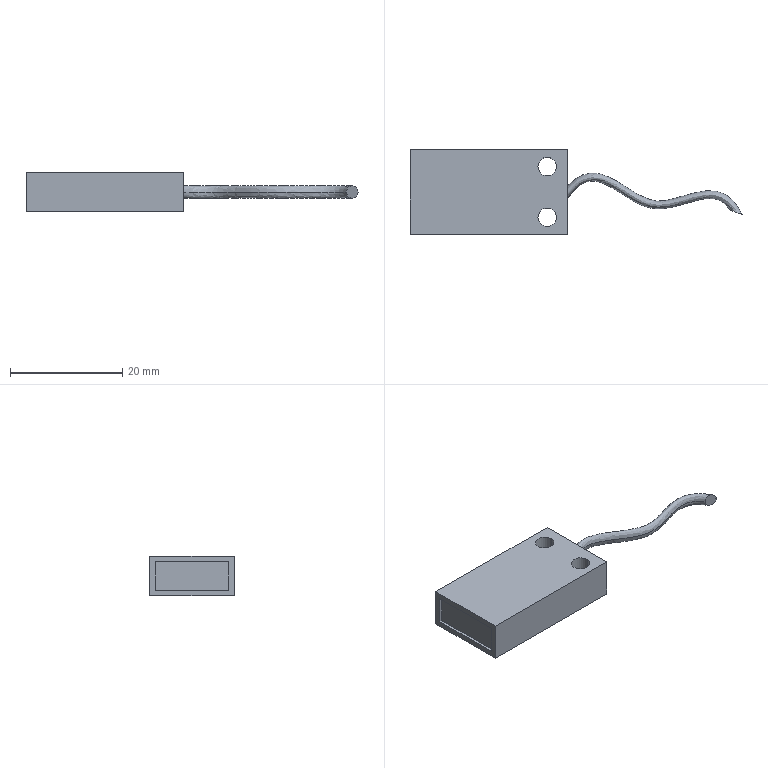Part | SolidWorks | features Extrusion 1, ICE 1, Sweep 1 | 1 solid | 18 faces | box 59.032 x 15 x 7 mm | volume 2869 mm3 | plane 12 | cylinder 4 | spline 2 | commonest cylinder face diameters 3.3 x4
STEP:
#1=CARTESIAN_POINT('',(14.,1.1,0.));
#2=VERTEX_POINT('',#1);
#3=CARTESIAN_POINT('',(14.,-1.1,0.));
#4=VERTEX_POINT('',#3);
#5=CARTESIAN_POINT('',(14.,0.,0.));
#6=DIRECTION('',(1.,0.,0.));
#7=DIRECTION('',(0.,0.,-1.));
#8=AXIS2_PLACEMENT_3D('',#5,#6,#7);
#9=CIRCLE('',#8,1.1);
#10=EDGE_CURVE('',#2,#4,#9,.T.);
#11=ORIENTED_EDGE('',*,*,#10,.T.);
#12=CARTESIAN_POINT('',(42.968,-3.234,0.));
#13=VERTEX_POINT('',#12);
#14=CARTESIAN_POINT('',(14.,-1.1,0.));
#15=CARTESIAN_POINT('',(14.23,-0.7808,0.));
#16=CARTESIAN_POINT('',(14.685,-0.2108,0.));
#17=CARTESIAN_POINT('',(15.325,0.4741,0.));
#18=CARTESIAN_POINT('',(15.935,1.009,0.));
#19=CARTESIAN_POINT('',(16.526,1.417,0.));
#20=CARTESIAN_POINT('',(17.248,1.776,0.));
#21=CARTESIAN_POINT('',(18.139,1.988,0.));
#22=CARTESIAN_POINT('',(19.247,1.912,0.));
#23=CARTESIAN_POINT('',(21.175,1.302,0.));
#24=CARTESIAN_POINT('',(23.958,-0.5364,0.));
#25=CARTESIAN_POINT('',(26.634,-2.268,0.));
#26=CARTESIAN_POINT('',(28.981,-2.948,0.));
#27=CARTESIAN_POINT('',(30.957,-3.112,0.));
#28=CARTESIAN_POINT('',(33.606,-2.495,0.));
#29=CARTESIAN_POINT('',(35.845,-1.781,0.));
#30=CARTESIAN_POINT('',(37.49,-1.354,0.));
#31=CARTESIAN_POINT('',(38.643,-1.156,0.));
#32=CARTESIAN_POINT('',(39.587,-1.126,0.));
#33=CARTESIAN_POINT('',(40.379,-1.248,0.));
#34=CARTESIAN_POINT('',(41.033,-1.47,0.));
#35=CARTESIAN_POINT('',(41.691,-1.851,0.));
#36=CARTESIAN_POINT('',(42.342,-2.418,0.));
#37=CARTESIAN_POINT('',(42.763,-2.94,0.));
#38=CARTESIAN_POINT('',(42.968,-3.234,0.));
#39=B_SPLINE_CURVE_WITH_KNOTS('',3,(#14,#15,#16,#17,#18,#19,#20,#21,#22,#23,#24,#25,#26,#27,#28,#29,#30,#31,#32,#33,#34,#35,#36,#37,#38),.UNSPECIFIED.,.F.,.F.,(4,1,1,1,1,1,1,1,1,1,1,1,1,1,1,1,1,1,1,1,1,1,4),(0.,0.025,0.05,0.075,0.1,0.125,0.1667,0.2083,0.25,0.375,0.5,0.5186,0.5833,0.6667,0.75,0.7917,0.8333,0.875,0.9,0.925,0.95,0.975,1.),.UNSPECIFIED.);
#40=EDGE_CURVE('',#4,#13,#39,.T.);
#41=ORIENTED_EDGE('',*,*,#40,.T.);
#42=CARTESIAN_POINT('',(45.032,-3.996,0.));
#43=VERTEX_POINT('',#42);
#44=CARTESIAN_POINT('',(44.,-3.615,0.));
#45=DIRECTION('',(0.3462,0.9382,0.));
#46=DIRECTION('',(-0.9382,0.3462,0.));
#47=AXIS2_PLACEMENT_3D('',#44,#45,#46);
#48=CIRCLE('',#47,1.1);
#49=EDGE_CURVE('',#13,#43,#48,.T.);
#50=ORIENTED_EDGE('',*,*,#49,.T.);
#51=CARTESIAN_POINT('',(14.,1.1,0.));
#52=CARTESIAN_POINT('',(14.304,1.417,0.));
#53=CARTESIAN_POINT('',(14.908,1.983,0.));
#54=CARTESIAN_POINT('',(15.828,2.623,0.));
#55=CARTESIAN_POINT('',(16.752,3.062,0.));
#56=CARTESIAN_POINT('',(17.672,3.307,0.));
#57=CARTESIAN_POINT('',(18.773,3.39,0.));
#58=CARTESIAN_POINT('',(20.003,3.198,0.));
#59=CARTESIAN_POINT('',(21.31,2.707,0.));
#60=CARTESIAN_POINT('',(23.372,1.619,0.));
#61=CARTESIAN_POINT('',(26.139,-0.3831,0.));
#62=CARTESIAN_POINT('',(28.781,-1.556,0.));
#63=CARTESIAN_POINT('',(30.762,-1.662,0.));
#64=CARTESIAN_POINT('',(32.352,-1.364,0.));
#65=CARTESIAN_POINT('',(34.786,-0.6503,0.));
#66=CARTESIAN_POINT('',(37.097,0.03487,0.));
#67=CARTESIAN_POINT('',(38.981,0.2719,0.));
#68=CARTESIAN_POINT('',(40.395,0.2,0.));
#69=CARTESIAN_POINT('',(41.586,-0.1671,0.));
#70=CARTESIAN_POINT('',(42.526,-0.7182,0.));
#71=CARTESIAN_POINT('',(43.238,-1.315,0.));
#72=CARTESIAN_POINT('',(43.89,-2.053,0.));
#73=CARTESIAN_POINT('',(44.488,-2.935,0.));
#74=CARTESIAN_POINT('',(44.855,-3.62,0.));
#75=CARTESIAN_POINT('',(45.032,-3.996,0.));
#76=B_SPLINE_CURVE_WITH_KNOTS('',3,(#51,#52,#53,#54,#55,#56,#57,#58,#59,#60,#61,#62,#63,#64,#65,#66,#67,#68,#69,#70,#71,#72,#73,#74,#75),.UNSPECIFIED.,.F.,.F.,(4,1,1,1,1,1,1,1,1,1,1,1,1,1,1,1,1,1,1,1,1,1,4),(0.,0.025,0.05,0.075,0.1,0.125,0.1667,0.2083,0.25,0.375,0.5,0.5186,0.5833,0.6667,0.75,0.7917,0.8333,0.875,0.9,0.925,0.95,0.975,1.),.UNSPECIFIED.);
#77=EDGE_CURVE('',#2,#43,#76,.T.);
#78=ORIENTED_EDGE('',*,*,#77,.F.);
#79=EDGE_LOOP('',(#11,#41,#50,#78));
#80=FACE_OUTER_BOUND('',#79,.T.);
#81=CARTESIAN_POINT('',(14.,1.1,0.));
#82=CARTESIAN_POINT('',(14.304,1.417,0.));
#83=CARTESIAN_POINT('',(14.908,1.983,0.));
#84=CARTESIAN_POINT('',(15.828,2.623,0.));
#85=CARTESIAN_POINT('',(16.752,3.062,0.));
#86=CARTESIAN_POINT('',(17.672,3.307,0.));
#87=CARTESIAN_POINT('',(18.773,3.39,0.));
#88=CARTESIAN_POINT('',(20.003,3.198,0.));
#89=CARTESIAN_POINT('',(21.31,2.707,0.));
#90=CARTESIAN_POINT('',(23.372,1.619,0.));
#91=CARTESIAN_POINT('',(26.139,-0.3831,0.));
#92=CARTESIAN_POINT('',(28.781,-1.556,0.));
#93=CARTESIAN_POINT('',(30.762,-1.662,0.));
#94=CARTESIAN_POINT('',(32.352,-1.364,0.));
#95=CARTESIAN_POINT('',(34.786,-0.6503,0.));
#96=CARTESIAN_POINT('',(37.097,0.03487,0.));
#97=CARTESIAN_POINT('',(38.981,0.2719,0.));
#98=CARTESIAN_POINT('',(40.395,0.2,0.));
#99=CARTESIAN_POINT('',(41.586,-0.1671,0.));
#100=CARTESIAN_POINT('',(42.526,-0.7182,0.));
#101=CARTESIAN_POINT('',(43.238,-1.315,0.));
#102=CARTESIAN_POINT('',(43.89,-2.053,0.));
#103=CARTESIAN_POINT('',(44.488,-2.935,0.));
#104=CARTESIAN_POINT('',(44.855,-3.62,0.));
#105=CARTESIAN_POINT('',(45.032,-3.996,0.));
#106=CARTESIAN_POINT('',(14.,1.1,2.2));
#107=CARTESIAN_POINT('',(14.304,1.417,2.2));
#108=CARTESIAN_POINT('',(14.908,1.983,2.2));
#109=CARTESIAN_POINT('',(15.828,2.623,2.2));
#110=CARTESIAN_POINT('',(16.752,3.062,2.2));
#111=CARTESIAN_POINT('',(17.672,3.307,2.2));
#112=CARTESIAN_POINT('',(18.773,3.39,2.2));
#113=CARTESIAN_POINT('',(20.003,3.198,2.2));
#114=CARTESIAN_POINT('',(21.31,2.707,2.2));
#115=CARTESIAN_POINT('',(23.372,1.619,2.2));
#116=CARTESIAN_POINT('',(26.139,-0.3831,2.2));
#117=CARTESIAN_POINT('',(28.781,-1.556,2.2));
#118=CARTESIAN_POINT('',(30.762,-1.662,2.2));
#119=CARTESIAN_POINT('',(32.352,-1.364,2.2));
#120=CARTESIAN_POINT('',(34.786,-0.6503,2.2));
#121=CARTESIAN_POINT('',(37.097,0.03487,2.2));
#122=CARTESIAN_POINT('',(38.981,0.2719,2.2));
#123=CARTESIAN_POINT('',(40.395,0.2,2.2));
#124=CARTESIAN_POINT('',(41.586,-0.1671,2.2));
#125=CARTESIAN_POINT('',(42.526,-0.7182,2.2));
#126=CARTESIAN_POINT('',(43.238,-1.315,2.2));
#127=CARTESIAN_POINT('',(43.89,-2.053,2.2));
#128=CARTESIAN_POINT('',(44.488,-2.935,2.2));
#129=CARTESIAN_POINT('',(44.855,-3.62,2.2));
#130=CARTESIAN_POINT('',(45.032,-3.996,2.2));
#131=CARTESIAN_POINT('',(14.,-1.1,2.2));
#132=CARTESIAN_POINT('',(14.23,-0.7808,2.2));
#133=CARTESIAN_POINT('',(14.685,-0.2108,2.2));
#134=CARTESIAN_POINT('',(15.325,0.4741,2.2));
#135=CARTESIAN_POINT('',(15.935,1.009,2.2));
#136=CARTESIAN_POINT('',(16.526,1.417,2.2));
#137=CARTESIAN_POINT('',(17.248,1.776,2.2));
#138=CARTESIAN_POINT('',(18.139,1.988,2.2));
#139=CARTESIAN_POINT('',(19.247,1.912,2.2));
#140=CARTESIAN_POINT('',(21.175,1.302,2.2));
#141=CARTESIAN_POINT('',(23.958,-0.5364,2.2));
#142=CARTESIAN_POINT('',(26.634,-2.268,2.2));
#143=CARTESIAN_POINT('',(28.981,-2.948,2.2));
#144=CARTESIAN_POINT('',(30.957,-3.112,2.2));
#145=CARTESIAN_POINT('',(33.606,-2.495,2.2));
#146=CARTESIAN_POINT('',(35.845,-1.781,2.2));
#147=CARTESIAN_POINT('',(37.49,-1.354,2.2));
#148=CARTESIAN_POINT('',(38.643,-1.156,2.2));
#149=CARTESIAN_POINT('',(39.587,-1.126,2.2));
#150=CARTESIAN_POINT('',(40.379,-1.248,2.2));
#151=CARTESIAN_POINT('',(41.033,-1.47,2.2));
#152=CARTESIAN_POINT('',(41.691,-1.851,2.2));
#153=CARTESIAN_POINT('',(42.342,-2.418,2.2));
#154=CARTESIAN_POINT('',(42.763,-2.94,2.2));
#155=CARTESIAN_POINT('',(42.968,-3.234,2.2));
#156=CARTESIAN_POINT('',(14.,-1.1,0.));
#157=CARTESIAN_POINT('',(14.23,-0.7808,0.));
#158=CARTESIAN_POINT('',(14.685,-0.2108,0.));
#159=CARTESIAN_POINT('',(15.325,0.4741,0.));
#160=CARTESIAN_POINT('',(15.935,1.009,0.));
#161=CARTESIAN_POINT('',(16.526,1.417,0.));
#162=CARTESIAN_POINT('',(17.248,1.776,0.));
#163=CARTESIAN_POINT('',(18.139,1.988,0.));
#164=CARTESIAN_POINT('',(19.247,1.912,0.));
#165=CARTESIAN_POINT('',(21.175,1.302,0.));
#166=CARTESIAN_POINT('',(23.958,-0.5364,0.));
#167=CARTESIAN_POINT('',(26.634,-2.268,0.));
#168=CARTESIAN_POINT('',(28.981,-2.948,0.));
#169=CARTESIAN_POINT('',(30.957,-3.112,0.));
#170=CARTESIAN_POINT('',(33.606,-2.495,0.));
#171=CARTESIAN_POINT('',(35.845,-1.781,0.));
#172=CARTESIAN_POINT('',(37.49,-1.354,0.));
#173=CARTESIAN_POINT('',(38.643,-1.156,0.));
#174=CARTESIAN_POINT('',(39.587,-1.126,0.));
#175=CARTESIAN_POINT('',(40.379,-1.248,0.));
#176=CARTESIAN_POINT('',(41.033,-1.47,0.));
#177=CARTESIAN_POINT('',(41.691,-1.851,0.));
#178=CARTESIAN_POINT('',(42.342,-2.418,0.));
#179=CARTESIAN_POINT('',(42.763,-2.94,0.));
#180=CARTESIAN_POINT('',(42.968,-3.234,0.));
#181=CARTESIAN_POINT('',(14.,-1.1,-2.2));
#182=CARTESIAN_POINT('',(14.23,-0.7808,-2.2));
#183=CARTESIAN_POINT('',(14.685,-0.2108,-2.2));
#184=CARTESIAN_POINT('',(15.325,0.4741,-2.2));
#185=CARTESIAN_POINT('',(15.935,1.009,-2.2));
#186=CARTESIAN_POINT('',(16.526,1.417,-2.2));
#187=CARTESIAN_POINT('',(17.248,1.776,-2.2));
#188=CARTESIAN_POINT('',(18.139,1.988,-2.2));
#189=CARTESIAN_POINT('',(19.247,1.912,-2.2));
#190=CARTESIAN_POINT('',(21.175,1.302,-2.2));
#191=CARTESIAN_POINT('',(23.958,-0.5364,-2.2));
#192=CARTESIAN_POINT('',(26.634,-2.268,-2.2));
#193=CARTESIAN_POINT('',(28.981,-2.948,-2.2));
#194=CARTESIAN_POINT('',(30.957,-3.112,-2.2));
#195=CARTESIAN_POINT('',(33.606,-2.495,-2.2));
#196=CARTESIAN_POINT('',(35.845,-1.781,-2.2));
#197=CARTESIAN_POINT('',(37.49,-1.354,-2.2));
#198=CARTESIAN_POINT('',(38.643,-1.156,-2.2));
#199=CARTESIAN_POINT('',(39.587,-1.126,-2.2));
#200=CARTESIAN_POINT('',(40.379,-1.248,-2.2));
#201=CARTESIAN_POINT('',(41.033,-1.47,-2.2));
#202=CARTESIAN_POINT('',(41.691,-1.851,-2.2));
#203=CARTESIAN_POINT('',(42.342,-2.418,-2.2));
#204=CARTESIAN_POINT('',(42.763,-2.94,-2.2));
#205=CARTESIAN_POINT('',(42.968,-3.234,-2.2));
#206=CARTESIAN_POINT('',(14.,1.1,-2.2));
#207=CARTESIAN_POINT('',(14.304,1.417,-2.2));
#208=CARTESIAN_POINT('',(14.908,1.983,-2.2));
#209=CARTESIAN_POINT('',(15.828,2.623,-2.2));
#210=CARTESIAN_POINT('',(16.752,3.062,-2.2));
#211=CARTESIAN_POINT('',(17.672,3.307,-2.2));
#212=CARTESIAN_POINT('',(18.773,3.39,-2.2));
#213=CARTESIAN_POINT('',(20.003,3.198,-2.2));
#214=CARTESIAN_POINT('',(21.31,2.707,-2.2));
#215=CARTESIAN_POINT('',(23.372,1.619,-2.2));
#216=CARTESIAN_POINT('',(26.139,-0.3831,-2.2));
#217=CARTESIAN_POINT('',(28.781,-1.556,-2.2));
#218=CARTESIAN_POINT('',(30.762,-1.662,-2.2));
#219=CARTESIAN_POINT('',(32.352,-1.364,-2.2));
#220=CARTESIAN_POINT('',(34.786,-0.6503,-2.2));
#221=CARTESIAN_POINT('',(37.097,0.03487,-2.2));
#222=CARTESIAN_POINT('',(38.981,0.2719,-2.2));
#223=CARTESIAN_POINT('',(40.395,0.2,-2.2));
#224=CARTESIAN_POINT('',(41.586,-0.1671,-2.2));
#225=CARTESIAN_POINT('',(42.526,-0.7182,-2.2));
#226=CARTESIAN_POINT('',(43.238,-1.315,-2.2));
#227=CARTESIAN_POINT('',(43.89,-2.053,-2.2));
#228=CARTESIAN_POINT('',(44.488,-2.935,-2.2));
#229=CARTESIAN_POINT('',(44.855,-3.62,-2.2));
#230=CARTESIAN_POINT('',(45.032,-3.996,-2.2));
#231=CARTESIAN_POINT('',(14.,1.1,0.));
#232=CARTESIAN_POINT('',(14.304,1.417,0.));
#233=CARTESIAN_POINT('',(14.908,1.983,0.));
#234=CARTESIAN_POINT('',(15.828,2.623,0.));
#235=CARTESIAN_POINT('',(16.752,3.062,0.));
#236=CARTESIAN_POINT('',(17.672,3.307,0.));
#237=CARTESIAN_POINT('',(18.773,3.39,0.));
#238=CARTESIAN_POINT('',(20.003,3.198,0.));
#239=CARTESIAN_POINT('',(21.31,2.707,0.));
#240=CARTESIAN_POINT('',(23.372,1.619,0.));
#241=CARTESIAN_POINT('',(26.139,-0.3831,0.));
#242=CARTESIAN_POINT('',(28.781,-1.556,0.));
#243=CARTESIAN_POINT('',(30.762,-1.662,0.));
#244=CARTESIAN_POINT('',(32.352,-1.364,0.));
#245=CARTESIAN_POINT('',(34.786,-0.6503,0.));
#246=CARTESIAN_POINT('',(37.097,0.03487,0.));
#247=CARTESIAN_POINT('',(38.981,0.2719,0.));
#248=CARTESIAN_POINT('',(40.395,0.2,0.));
#249=CARTESIAN_POINT('',(41.586,-0.1671,0.));
#250=CARTESIAN_POINT('',(42.526,-0.7182,0.));
#251=CARTESIAN_POINT('',(43.238,-1.315,0.));
#252=CARTESIAN_POINT('',(43.89,-2.053,0.));
#253=CARTESIAN_POINT('',(44.488,-2.935,0.));
#254=CARTESIAN_POINT('',(44.855,-3.62,0.));
#255=CARTESIAN_POINT('',(45.032,-3.996,0.));
#256=(BOUNDED_SURFACE()B_SPLINE_SURFACE(3,3,((#81,#82,#83,#84,#85,#86,#87,#88,#89,#90,#91,#92,#93,#94,#95,#96,#97,#98,#99,#100,#101,#102,#103,#104,#105),(#106,#107,#108,#109,#110,#111,#112,#113,#114,#115,#116,#117,#118,#119,#120,#121,#122,#123,#124,#125,#126,#127,#128,#129,#130),(#131,#132,#133,#134,#135,#136,#137,#138,#139,#140,#141,#142,#143,#144,#145,#146,#147,#148,#149,#150,#151,#152,#153,#154,#155),(#156,#157,#158,#159,#160,#161,#162,#163,#164,#165,#166,#167,#168,#169,#170,#171,#172,#173,#174,#175,#176,#177,#178,#179,#180),(#181,#182,#183,#184,#185,#186,#187,#188,#189,#190,#191,#192,#193,#194,#195,#196,#197,#198,#199,#200,#201,#202,#203,#204,#205),(#206,#207,#208,#209,#210,#211,#212,#213,#214,#215,#216,#217,#218,#219,#220,#221,#222,#223,#224,#225,#226,#227,#228,#229,#230),(#231,#232,#233,#234,#235,#236,#237,#238,#239,#240,#241,#242,#243,#244,#245,#246,#247,#248,#249,#250,#251,#252,#253,#254,#255)),.UNSPECIFIED.,.T.,.F.,.F.)B_SPLINE_SURFACE_WITH_KNOTS((4,3,4),(4,1,1,1,1,1,1,1,1,1,1,1,1,1,1,1,1,1,1,1,1,1,4),(0.,0.5,1.),(0.,0.025,0.05,0.075,0.1,0.125,0.1667,0.2083,0.25,0.375,0.5,0.5186,0.5833,0.6667,0.75,0.7917,0.8333,0.875,0.9,0.925,0.95,0.975,1.),.UNSPECIFIED.)GEOMETRIC_REPRESENTATION_ITEM()RATIONAL_B_SPLINE_SURFACE(((1.,1.,1.,1.,1.,1.,1.,1.,1.,1.,1.,1.,1.,1.,1.,1.,1.,1.,1.,1.,1.,1.,1.,1.,1.),(0.3333,0.3333,0.3333,0.3333,0.3333,0.3333,0.3333,0.3333,0.3333,0.3333,0.3333,0.3333,0.3333,0.3333,0.3333,0.3333,0.3333,0.3333,0.3333,0.3333,0.3333,0.3333,0.3333,0.3333,0.3333),(0.3333,0.3333,0.3333,0.3333,0.3333,0.3333,0.3333,0.3333,0.3333,0.3333,0.3333,0.3333,0.3333,0.3333,0.3333,0.3333,0.3333,0.3333,0.3333,0.3333,0.3333,0.3333,0.3333,0.3333,0.3333),(1.,1.,1.,1.,1.,1.,1.,1.,1.,1.,1.,1.,1.,1.,1.,1.,1.,1.,1.,1.,1.,1.,1.,1.,1.),(0.3333,0.3333,0.3333,0.3333,0.3333,0.3333,0.3333,0.3333,0.3333,0.3333,0.3333,0.3333,0.3333,0.3333,0.3333,0.3333,0.3333,0.3333,0.3333,0.3333,0.3333,0.3333,0.3333,0.3333,0.3333),(0.3333,0.3333,0.3333,0.3333,0.3333,0.3333,0.3333,0.3333,0.3333,0.3333,0.3333,0.3333,0.3333,0.3333,0.3333,0.3333,0.3333,0.3333,0.3333,0.3333,0.3333,0.3333,0.3333,0.3333,0.3333),(1.,1.,1.,1.,1.,1.,1.,1.,1.,1.,1.,1.,1.,1.,1.,1.,1.,1.,1.,1.,1.,1.,1.,1.,1.)))REPRESENTATION_ITEM('')SURFACE());
#257=ADVANCED_FACE('',(#80),#256,.T.);
#258=CARTESIAN_POINT('',(8.75,-4.5,3.5));
#259=VERTEX_POINT('',#258);
#260=CARTESIAN_POINT('',(12.05,-4.5,3.5));
#261=VERTEX_POINT('',#260);
#262=CARTESIAN_POINT('',(10.4,-4.5,3.5));
#263=DIRECTION('',(0.,0.,1.));
#264=DIRECTION('',(1.,0.,0.));
#265=AXIS2_PLACEMENT_3D('',#262,#263,#264);
#266=CIRCLE('',#265,1.65);
#267=EDGE_CURVE('',#259,#261,#266,.T.);
#268=ORIENTED_EDGE('',*,*,#267,.T.);
#269=CARTESIAN_POINT('',(12.05,-4.5,-3.5));
#270=VERTEX_POINT('',#269);
#271=CARTESIAN_POINT('',(12.05,-4.5,3.5));
#272=DIRECTION('',(0.,0.,-1.));
#273=VECTOR('',#272,1000.);
#274=LINE('',#271,#273);
#275=EDGE_CURVE('',#261,#270,#274,.T.);
#276=ORIENTED_EDGE('',*,*,#275,.T.);
#277=CARTESIAN_POINT('',(8.75,-4.5,-3.5));
#278=VERTEX_POINT('',#277);
#279=CARTESIAN_POINT('',(10.4,-4.5,-3.5));
#280=DIRECTION('',(0.,0.,1.));
#281=DIRECTION('',(1.,0.,0.));
#282=AXIS2_PLACEMENT_3D('',#279,#280,#281);
#283=CIRCLE('',#282,1.65);
#284=EDGE_CURVE('',#278,#270,#283,.T.);
#285=ORIENTED_EDGE('',*,*,#284,.F.);
#286=CARTESIAN_POINT('',(8.75,-4.5,3.5));
#287=DIRECTION('',(0.,0.,-1.));
#288=VECTOR('',#287,1000.);
#289=LINE('',#286,#288);
#290=EDGE_CURVE('',#259,#278,#289,.T.);
#291=ORIENTED_EDGE('',*,*,#290,.F.);
#292=EDGE_LOOP('',(#268,#276,#285,#291));
#293=FACE_OUTER_BOUND('',#292,.T.);
#294=CARTESIAN_POINT('',(10.4,-4.5,3.5));
#295=DIRECTION('',(0.,0.,-1.));
#296=DIRECTION('',(-1.,0.,0.));
#297=AXIS2_PLACEMENT_3D('',#294,#295,#296);
#298=CYLINDRICAL_SURFACE('',#297,1.65);
#299=ADVANCED_FACE('',(#293),#298,.F.);
#300=CARTESIAN_POINT('',(8.75,4.5,3.5));
#301=VERTEX_POINT('',#300);
#302=CARTESIAN_POINT('',(12.05,4.5,3.5));
#303=VERTEX_POINT('',#302);
#304=CARTESIAN_POINT('',(10.4,4.5,3.5));
#305=DIRECTION('',(0.,0.,1.));
#306=DIRECTION('',(1.,0.,0.));
#307=AXIS2_PLACEMENT_3D('',#304,#305,#306);
#308=CIRCLE('',#307,1.65);
#309=EDGE_CURVE('',#301,#303,#308,.T.);
#310=ORIENTED_EDGE('',*,*,#309,.T.);
#311=CARTESIAN_POINT('',(12.05,4.5,-3.5));
#312=VERTEX_POINT('',#311);
#313=CARTESIAN_POINT('',(12.05,4.5,3.5));
#314=DIRECTION('',(0.,0.,-1.));
#315=VECTOR('',#314,1000.);
#316=LINE('',#313,#315);
#317=EDGE_CURVE('',#303,#312,#316,.T.);
#318=ORIENTED_EDGE('',*,*,#317,.T.);
#319=CARTESIAN_POINT('',(8.75,4.5,-3.5));
#320=VERTEX_POINT('',#319);
#321=CARTESIAN_POINT('',(10.4,4.5,-3.5));
#322=DIRECTION('',(0.,0.,1.));
#323=DIRECTION('',(1.,0.,0.));
#324=AXIS2_PLACEMENT_3D('',#321,#322,#323);
#325=CIRCLE('',#324,1.65);
#326=EDGE_CURVE('',#320,#312,#325,.T.);
#327=ORIENTED_EDGE('',*,*,#326,.F.);
#328=CARTESIAN_POINT('',(8.75,4.5,3.5));
#329=DIRECTION('',(0.,0.,-1.));
#330=VECTOR('',#329,1000.);
#331=LINE('',#328,#330);
#332=EDGE_CURVE('',#301,#320,#331,.T.);
#333=ORIENTED_EDGE('',*,*,#332,.F.);
#334=EDGE_LOOP('',(#310,#318,#327,#333));
#335=FACE_OUTER_BOUND('',#334,.T.);
#336=CARTESIAN_POINT('',(10.4,4.5,3.5));
#337=DIRECTION('',(0.,0.,-1.));
#338=DIRECTION('',(-1.,0.,0.));
#339=AXIS2_PLACEMENT_3D('',#336,#337,#338);
#340=CYLINDRICAL_SURFACE('',#339,1.65);
#341=ADVANCED_FACE('',(#335),#340,.F.);
#342=CARTESIAN_POINT('',(14.,-7.5,-3.5));
#343=VERTEX_POINT('',#342);
#344=CARTESIAN_POINT('',(14.,7.5,-3.5));
#345=VERTEX_POINT('',#344);
#346=CARTESIAN_POINT('',(14.,7.5,-3.5));
#347=DIRECTION('',(0.,1.,0.));
#348=VECTOR('',#347,1000.);
#349=LINE('',#346,#348);
#350=EDGE_CURVE('',#343,#345,#349,.T.);
#351=ORIENTED_EDGE('',*,*,#350,.T.);
#352=CARTESIAN_POINT('',(14.,7.5,3.5));
#353=VERTEX_POINT('',#352);
#354=CARTESIAN_POINT('',(14.,7.5,3.5));
#355=DIRECTION('',(0.,0.,-1.));
#356=VECTOR('',#355,1000.);
#357=LINE('',#354,#356);
#358=EDGE_CURVE('',#353,#345,#357,.T.);
#359=ORIENTED_EDGE('',*,*,#358,.F.);
#360=CARTESIAN_POINT('',(14.,-7.5,3.5));
#361=VERTEX_POINT('',#360);
#362=CARTESIAN_POINT('',(14.,7.5,3.5));
#363=DIRECTION('',(0.,1.,0.));
#364=VECTOR('',#363,1000.);
#365=LINE('',#362,#364);
#366=EDGE_CURVE('',#361,#353,#365,.T.);
#367=ORIENTED_EDGE('',*,*,#366,.F.);
#368=CARTESIAN_POINT('',(14.,-7.5,3.5));
#369=DIRECTION('',(0.,0.,-1.));
#370=VECTOR('',#369,1000.);
#371=LINE('',#368,#370);
#372=EDGE_CURVE('',#361,#343,#371,.T.);
#373=ORIENTED_EDGE('',*,*,#372,.T.);
#374=EDGE_LOOP('',(#351,#359,#367,#373));
#375=FACE_OUTER_BOUND('',#374,.T.);
#376=ORIENTED_EDGE('',*,*,#10,.F.);
#377=CARTESIAN_POINT('',(14.,0.,0.));
#378=DIRECTION('',(1.,0.,0.));
#379=DIRECTION('',(0.,0.,-1.));
#380=AXIS2_PLACEMENT_3D('',#377,#378,#379);
#381=CIRCLE('',#380,1.1);
#382=EDGE_CURVE('',#4,#2,#381,.T.);
#383=ORIENTED_EDGE('',*,*,#382,.F.);
#384=EDGE_LOOP('',(#376,#383));
#385=FACE_BOUND('',#384,.T.);
#386=CARTESIAN_POINT('',(14.,7.5,3.5));
#387=DIRECTION('',(-1.,0.,0.));
#388=DIRECTION('',(0.,-1.,0.));
#389=AXIS2_PLACEMENT_3D('',#386,#387,#388);
#390=PLANE('',#389);
#391=ADVANCED_FACE('',(#375,#385),#390,.F.);
#392=ORIENTED_EDGE('',*,*,#309,.F.);
#393=CARTESIAN_POINT('',(10.4,4.5,3.5));
#394=DIRECTION('',(0.,0.,1.));
#395=DIRECTION('',(1.,0.,0.));
#396=AXIS2_PLACEMENT_3D('',#393,#394,#395);
#397=CIRCLE('',#396,1.65);
#398=EDGE_CURVE('',#303,#301,#397,.T.);
#399=ORIENTED_EDGE('',*,*,#398,.F.);
#400=EDGE_LOOP('',(#392,#399));
#401=FACE_BOUND('',#400,.T.);
#402=CARTESIAN_POINT('',(-14.,7.5,3.5));
#403=VERTEX_POINT('',#402);
#404=CARTESIAN_POINT('',(-14.,-7.5,3.5));
#405=VERTEX_POINT('',#404);
#406=CARTESIAN_POINT('',(-14.,7.5,3.5));
#407=DIRECTION('',(0.,-1.,0.));
#408=VECTOR('',#407,1000.);
#409=LINE('',#406,#408);
#410=EDGE_CURVE('',#403,#405,#409,.T.);
#411=ORIENTED_EDGE('',*,*,#410,.T.);
#412=CARTESIAN_POINT('',(-14.,-7.5,3.5));
#413=DIRECTION('',(1.,0.,0.));
#414=VECTOR('',#413,1000.);
#415=LINE('',#412,#414);
#416=EDGE_CURVE('',#405,#361,#415,.T.);
#417=ORIENTED_EDGE('',*,*,#416,.T.);
#418=ORIENTED_EDGE('',*,*,#366,.T.);
#419=CARTESIAN_POINT('',(-14.,7.5,3.5));
#420=DIRECTION('',(-1.,0.,0.));
#421=VECTOR('',#420,1000.);
#422=LINE('',#419,#421);
#423=EDGE_CURVE('',#353,#403,#422,.T.);
#424=ORIENTED_EDGE('',*,*,#423,.T.);
#425=EDGE_LOOP('',(#411,#417,#418,#424));
#426=FACE_OUTER_BOUND('',#425,.T.);
#427=ORIENTED_EDGE('',*,*,#267,.F.);
#428=CARTESIAN_POINT('',(10.4,-4.5,3.5));
#429=DIRECTION('',(0.,0.,1.));
#430=DIRECTION('',(1.,0.,0.));
#431=AXIS2_PLACEMENT_3D('',#428,#429,#430);
#432=CIRCLE('',#431,1.65);
#433=EDGE_CURVE('',#261,#259,#432,.T.);
#434=ORIENTED_EDGE('',*,*,#433,.F.);
#435=EDGE_LOOP('',(#427,#434));
#436=FACE_BOUND('',#435,.T.);
#437=CARTESIAN_POINT('',(-14.,-7.5,3.5));
#438=DIRECTION('',(0.,0.,1.));
#439=DIRECTION('',(1.,0.,0.));
#440=AXIS2_PLACEMENT_3D('',#437,#438,#439);
#441=PLANE('',#440);
#442=ADVANCED_FACE('',(#401,#426,#436),#441,.T.);
#443=ORIENTED_EDGE('',*,*,#326,.T.);
#444=CARTESIAN_POINT('',(10.4,4.5,-3.5));
#445=DIRECTION('',(0.,0.,1.));
#446=DIRECTION('',(1.,0.,0.));
#447=AXIS2_PLACEMENT_3D('',#444,#445,#446);
#448=CIRCLE('',#447,1.65);
#449=EDGE_CURVE('',#312,#320,#448,.T.);
#450=ORIENTED_EDGE('',*,*,#449,.T.);
#451=EDGE_LOOP('',(#443,#450));
#452=FACE_BOUND('',#451,.T.);
#453=CARTESIAN_POINT('',(-14.,7.5,-3.5));
#454=VERTEX_POINT('',#453);
#455=CARTESIAN_POINT('',(-14.,-7.5,-3.5));
#456=VERTEX_POINT('',#455);
#457=CARTESIAN_POINT('',(-14.,7.5,-3.5));
#458=DIRECTION('',(0.,-1.,0.));
#459=VECTOR('',#458,1000.);
#460=LINE('',#457,#459);
#461=EDGE_CURVE('',#454,#456,#460,.T.);
#462=ORIENTED_EDGE('',*,*,#461,.F.);
#463=CARTESIAN_POINT('',(-14.,7.5,-3.5));
#464=DIRECTION('',(-1.,0.,0.));
#465=VECTOR('',#464,1000.);
#466=LINE('',#463,#465);
#467=EDGE_CURVE('',#345,#454,#466,.T.);
#468=ORIENTED_EDGE('',*,*,#467,.F.);
#469=ORIENTED_EDGE('',*,*,#350,.F.);
#470=CARTESIAN_POINT('',(-14.,-7.5,-3.5));
#471=DIRECTION('',(1.,0.,0.));
#472=VECTOR('',#471,1000.);
#473=LINE('',#470,#472);
#474=EDGE_CURVE('',#456,#343,#473,.T.);
#475=ORIENTED_EDGE('',*,*,#474,.F.);
#476=EDGE_LOOP('',(#462,#468,#469,#475));
#477=FACE_OUTER_BOUND('',#476,.T.);
#478=ORIENTED_EDGE('',*,*,#284,.T.);
#479=CARTESIAN_POINT('',(10.4,-4.5,-3.5));
#480=DIRECTION('',(0.,0.,1.));
#481=DIRECTION('',(1.,0.,0.));
#482=AXIS2_PLACEMENT_3D('',#479,#480,#481);
#483=CIRCLE('',#482,1.65);
#484=EDGE_CURVE('',#270,#278,#483,.T.);
#485=ORIENTED_EDGE('',*,*,#484,.T.);
#486=EDGE_LOOP('',(#478,#485));
#487=FACE_BOUND('',#486,.T.);
#488=CARTESIAN_POINT('',(-14.,-7.5,-3.5));
#489=DIRECTION('',(0.,0.,1.));
#490=DIRECTION('',(1.,0.,0.));
#491=AXIS2_PLACEMENT_3D('',#488,#489,#490);
#492=PLANE('',#491);
#493=ADVANCED_FACE('',(#452,#477,#487),#492,.F.);
#494=CARTESIAN_POINT('',(-14.,-6.5,-2.5));
#495=VERTEX_POINT('',#494);
#496=CARTESIAN_POINT('',(-14.,-6.5,2.5));
#497=VERTEX_POINT('',#496);
#498=CARTESIAN_POINT('',(-14.,-6.5,-2.5));
#499=DIRECTION('',(0.,0.,1.));
#500=VECTOR('',#499,1000.);
#501=LINE('',#498,#500);
#502=EDGE_CURVE('',#495,#497,#501,.T.);
#503=ORIENTED_EDGE('',*,*,#502,.F.);
#504=CARTESIAN_POINT('',(-14.,6.5,-2.5));
#505=VERTEX_POINT('',#504);
#506=CARTESIAN_POINT('',(-14.,6.5,-2.5));
#507=DIRECTION('',(0.,-1.,0.));
#508=VECTOR('',#507,1000.);
#509=LINE('',#506,#508);
#510=EDGE_CURVE('',#505,#495,#509,.T.);
#511=ORIENTED_EDGE('',*,*,#510,.F.);
#512=CARTESIAN_POINT('',(-14.,6.5,2.5));
#513=VERTEX_POINT('',#512);
#514=CARTESIAN_POINT('',(-14.,6.5,-2.5));
#515=DIRECTION('',(0.,0.,-1.));
#516=VECTOR('',#515,1000.);
#517=LINE('',#514,#516);
#518=EDGE_CURVE('',#513,#505,#517,.T.);
#519=ORIENTED_EDGE('',*,*,#518,.F.);
#520=CARTESIAN_POINT('',(-14.,6.5,2.5));
#521=DIRECTION('',(0.,1.,0.));
#522=VECTOR('',#521,1000.);
#523=LINE('',#520,#522);
#524=EDGE_CURVE('',#497,#513,#523,.T.);
#525=ORIENTED_EDGE('',*,*,#524,.F.);
#526=EDGE_LOOP('',(#503,#511,#519,#525));
#527=FACE_BOUND('',#526,.T.);
#528=ORIENTED_EDGE('',*,*,#461,.T.);
#529=CARTESIAN_POINT('',(-14.,-7.5,3.5));
#530=DIRECTION('',(0.,0.,-1.));
#531=VECTOR('',#530,1000.);
#532=LINE('',#529,#531);
#533=EDGE_CURVE('',#405,#456,#532,.T.);
#534=ORIENTED_EDGE('',*,*,#533,.F.);
#535=ORIENTED_EDGE('',*,*,#410,.F.);
#536=CARTESIAN_POINT('',(-14.,7.5,3.5));
#537=DIRECTION('',(0.,0.,-1.));
#538=VECTOR('',#537,1000.);
#539=LINE('',#536,#538);
#540=EDGE_CURVE('',#403,#454,#539,.T.);
#541=ORIENTED_EDGE('',*,*,#540,.T.);
#542=EDGE_LOOP('',(#528,#534,#535,#541));
#543=FACE_OUTER_BOUND('',#542,.T.);
#544=CARTESIAN_POINT('',(-14.,7.5,3.5));
#545=DIRECTION('',(1.,0.,0.));
#546=DIRECTION('',(0.,0.,-1.));
#547=AXIS2_PLACEMENT_3D('',#544,#545,#546);
#548=PLANE('',#547);
#549=ADVANCED_FACE('',(#527,#543),#548,.F.);
#550=ORIENTED_EDGE('',*,*,#474,.T.);
#551=ORIENTED_EDGE('',*,*,#372,.F.);
#552=ORIENTED_EDGE('',*,*,#416,.F.);
#553=ORIENTED_EDGE('',*,*,#533,.T.);
#554=EDGE_LOOP('',(#550,#551,#552,#553));
#555=FACE_OUTER_BOUND('',#554,.T.);
#556=CARTESIAN_POINT('',(-14.,-7.5,3.5));
#557=DIRECTION('',(0.,1.,0.));
#558=DIRECTION('',(-1.,0.,0.));
#559=AXIS2_PLACEMENT_3D('',#556,#557,#558);
#560=PLANE('',#559);
#561=ADVANCED_FACE('',(#555),#560,.F.);
#562=ORIENTED_EDGE('',*,*,#467,.T.);
#563=ORIENTED_EDGE('',*,*,#540,.F.);
#564=ORIENTED_EDGE('',*,*,#423,.F.);
#565=ORIENTED_EDGE('',*,*,#358,.T.);
#566=EDGE_LOOP('',(#562,#563,#564,#565));
#567=FACE_OUTER_BOUND('',#566,.T.);
#568=CARTESIAN_POINT('',(-14.,7.5,3.5));
#569=DIRECTION('',(0.,-1.,0.));
#570=DIRECTION('',(0.,0.,-1.));
#571=AXIS2_PLACEMENT_3D('',#568,#569,#570);
#572=PLANE('',#571);
#573=ADVANCED_FACE('',(#567),#572,.F.);
#574=ORIENTED_EDGE('',*,*,#317,.F.);
#575=ORIENTED_EDGE('',*,*,#398,.T.);
#576=ORIENTED_EDGE('',*,*,#332,.T.);
#577=ORIENTED_EDGE('',*,*,#449,.F.);
#578=EDGE_LOOP('',(#574,#575,#576,#577));
#579=FACE_OUTER_BOUND('',#578,.T.);
#580=CARTESIAN_POINT('',(10.4,4.5,3.5));
#581=DIRECTION('',(0.,0.,-1.));
#582=DIRECTION('',(-1.,0.,0.));
#583=AXIS2_PLACEMENT_3D('',#580,#581,#582);
#584=CYLINDRICAL_SURFACE('',#583,1.65);
#585=ADVANCED_FACE('',(#579),#584,.F.);
#586=ORIENTED_EDGE('',*,*,#275,.F.);
#587=ORIENTED_EDGE('',*,*,#433,.T.);
#588=ORIENTED_EDGE('',*,*,#290,.T.);
#589=ORIENTED_EDGE('',*,*,#484,.F.);
#590=EDGE_LOOP('',(#586,#587,#588,#589));
#591=FACE_OUTER_BOUND('',#590,.T.);
#592=CARTESIAN_POINT('',(10.4,-4.5,3.5));
#593=DIRECTION('',(0.,0.,-1.));
#594=DIRECTION('',(-1.,0.,0.));
#595=AXIS2_PLACEMENT_3D('',#592,#593,#594);
#596=CYLINDRICAL_SURFACE('',#595,1.65);
#597=ADVANCED_FACE('',(#591),#596,.F.);
#598=ORIENTED_EDGE('',*,*,#510,.T.);
#599=CARTESIAN_POINT('',(-13.5,-6.5,-2.5));
#600=VERTEX_POINT('',#599);
#601=CARTESIAN_POINT('',(-13.5,-6.5,-2.5));
#602=DIRECTION('',(-1.,0.,0.));
#603=VECTOR('',#602,1000.);
#604=LINE('',#601,#603);
#605=EDGE_CURVE('',#600,#495,#604,.T.);
#606=ORIENTED_EDGE('',*,*,#605,.F.);
#607=CARTESIAN_POINT('',(-13.5,6.5,-2.5));
#608=VERTEX_POINT('',#607);
#609=CARTESIAN_POINT('',(-13.5,6.5,-2.5));
#610=DIRECTION('',(0.,-1.,0.));
#611=VECTOR('',#610,1000.);
#612=LINE('',#609,#611);
#613=EDGE_CURVE('',#608,#600,#612,.T.);
#614=ORIENTED_EDGE('',*,*,#613,.F.);
#615=CARTESIAN_POINT('',(-13.5,6.5,-2.5));
#616=DIRECTION('',(-1.,0.,0.));
#617=VECTOR('',#616,1000.);
#618=LINE('',#615,#617);
#619=EDGE_CURVE('',#608,#505,#618,.T.);
#620=ORIENTED_EDGE('',*,*,#619,.T.);
#621=EDGE_LOOP('',(#598,#606,#614,#620));
#622=FACE_OUTER_BOUND('',#621,.T.);
#623=CARTESIAN_POINT('',(-13.5,6.5,-2.5));
#624=DIRECTION('',(0.,0.,-1.));
#625=DIRECTION('',(0.,1.,0.));
#626=AXIS2_PLACEMENT_3D('',#623,#624,#625);
#627=PLANE('',#626);
#628=ADVANCED_FACE('',(#622),#627,.F.);
#629=ORIENTED_EDGE('',*,*,#518,.T.);
#630=ORIENTED_EDGE('',*,*,#619,.F.);
#631=CARTESIAN_POINT('',(-13.5,6.5,2.5));
#632=VERTEX_POINT('',#631);
#633=CARTESIAN_POINT('',(-13.5,6.5,-2.5));
#634=DIRECTION('',(0.,0.,-1.));
#635=VECTOR('',#634,1000.);
#636=LINE('',#633,#635);
#637=EDGE_CURVE('',#632,#608,#636,.T.);
#638=ORIENTED_EDGE('',*,*,#637,.F.);
#639=CARTESIAN_POINT('',(-13.5,6.5,2.5));
#640=DIRECTION('',(-1.,0.,0.));
#641=VECTOR('',#640,1000.);
#642=LINE('',#639,#641);
#643=EDGE_CURVE('',#632,#513,#642,.T.);
#644=ORIENTED_EDGE('',*,*,#643,.T.);
#645=EDGE_LOOP('',(#629,#630,#638,#644));
#646=FACE_OUTER_BOUND('',#645,.T.);
#647=CARTESIAN_POINT('',(-13.5,6.5,-2.5));
#648=DIRECTION('',(0.,1.,0.));
#649=DIRECTION('',(0.,0.,1.));
#650=AXIS2_PLACEMENT_3D('',#647,#648,#649);
#651=PLANE('',#650);
#652=ADVANCED_FACE('',(#646),#651,.F.);
#653=ORIENTED_EDGE('',*,*,#524,.T.);
#654=ORIENTED_EDGE('',*,*,#643,.F.);
#655=CARTESIAN_POINT('',(-13.5,-6.5,2.5));
#656=VERTEX_POINT('',#655);
#657=CARTESIAN_POINT('',(-13.5,6.5,2.5));
#658=DIRECTION('',(0.,1.,0.));
#659=VECTOR('',#658,1000.);
#660=LINE('',#657,#659);
#661=EDGE_CURVE('',#656,#632,#660,.T.);
#662=ORIENTED_EDGE('',*,*,#661,.F.);
#663=CARTESIAN_POINT('',(-13.5,-6.5,2.5));
#664=DIRECTION('',(-1.,0.,0.));
#665=VECTOR('',#664,1000.);
#666=LINE('',#663,#665);
#667=EDGE_CURVE('',#656,#497,#666,.T.);
#668=ORIENTED_EDGE('',*,*,#667,.T.);
#669=EDGE_LOOP('',(#653,#654,#662,#668));
#670=FACE_OUTER_BOUND('',#669,.T.);
#671=CARTESIAN_POINT('',(-13.5,6.5,2.5));
#672=DIRECTION('',(0.,0.,1.));
#673=DIRECTION('',(0.,-1.,0.));
#674=AXIS2_PLACEMENT_3D('',#671,#672,#673);
#675=PLANE('',#674);
#676=ADVANCED_FACE('',(#670),#675,.F.);
#677=ORIENTED_EDGE('',*,*,#502,.T.);
#678=ORIENTED_EDGE('',*,*,#667,.F.);
#679=CARTESIAN_POINT('',(-13.5,-6.5,-2.5));
#680=DIRECTION('',(0.,0.,1.));
#681=VECTOR('',#680,1000.);
#682=LINE('',#679,#681);
#683=EDGE_CURVE('',#600,#656,#682,.T.);
#684=ORIENTED_EDGE('',*,*,#683,.F.);
#685=ORIENTED_EDGE('',*,*,#605,.T.);
#686=EDGE_LOOP('',(#677,#678,#684,#685));
#687=FACE_OUTER_BOUND('',#686,.T.);
#688=CARTESIAN_POINT('',(-13.5,-6.5,-2.5));
#689=DIRECTION('',(0.,-1.,0.));
#690=DIRECTION('',(0.,0.,-1.));
#691=AXIS2_PLACEMENT_3D('',#688,#689,#690);
#692=PLANE('',#691);
#693=ADVANCED_FACE('',(#687),#692,.F.);
#694=ORIENTED_EDGE('',*,*,#613,.T.);
#695=ORIENTED_EDGE('',*,*,#683,.T.);
#696=ORIENTED_EDGE('',*,*,#661,.T.);
#697=ORIENTED_EDGE('',*,*,#637,.T.);
#698=EDGE_LOOP('',(#694,#695,#696,#697));
#699=FACE_OUTER_BOUND('',#698,.T.);
#700=CARTESIAN_POINT('',(-13.5,-6.5,-2.5));
#701=DIRECTION('',(-1.,0.,0.));
#702=DIRECTION('',(0.,0.,1.));
#703=AXIS2_PLACEMENT_3D('',#700,#701,#702);
#704=PLANE('',#703);
#705=ADVANCED_FACE('',(#699),#704,.T.);
#706=ORIENTED_EDGE('',*,*,#40,.F.);
#707=ORIENTED_EDGE('',*,*,#382,.T.);
#708=ORIENTED_EDGE('',*,*,#77,.T.);
#709=CARTESIAN_POINT('',(44.,-3.615,0.));
#710=DIRECTION('',(0.3462,0.9382,0.));
#711=DIRECTION('',(-0.9382,0.3462,0.));
#712=AXIS2_PLACEMENT_3D('',#709,#710,#711);
#713=CIRCLE('',#712,1.1);
#714=EDGE_CURVE('',#43,#13,#713,.T.);
#715=ORIENTED_EDGE('',*,*,#714,.T.);
#716=EDGE_LOOP('',(#706,#707,#708,#715));
#717=FACE_OUTER_BOUND('',#716,.T.);
#718=CARTESIAN_POINT('',(14.,1.1,0.));
#719=CARTESIAN_POINT('',(14.304,1.417,0.));
#720=CARTESIAN_POINT('',(14.908,1.983,0.));
#721=CARTESIAN_POINT('',(15.828,2.623,0.));
#722=CARTESIAN_POINT('',(16.752,3.062,0.));
#723=CARTESIAN_POINT('',(17.672,3.307,0.));
#724=CARTESIAN_POINT('',(18.773,3.39,0.));
#725=CARTESIAN_POINT('',(20.003,3.198,0.));
#726=CARTESIAN_POINT('',(21.31,2.707,0.));
#727=CARTESIAN_POINT('',(23.372,1.619,0.));
#728=CARTESIAN_POINT('',(26.139,-0.3831,0.));
#729=CARTESIAN_POINT('',(28.781,-1.556,0.));
#730=CARTESIAN_POINT('',(30.762,-1.662,0.));
#731=CARTESIAN_POINT('',(32.352,-1.364,0.));
#732=CARTESIAN_POINT('',(34.786,-0.6503,0.));
#733=CARTESIAN_POINT('',(37.097,0.03487,0.));
#734=CARTESIAN_POINT('',(38.981,0.2719,0.));
#735=CARTESIAN_POINT('',(40.395,0.2,0.));
#736=CARTESIAN_POINT('',(41.586,-0.1671,0.));
#737=CARTESIAN_POINT('',(42.526,-0.7182,0.));
#738=CARTESIAN_POINT('',(43.238,-1.315,0.));
#739=CARTESIAN_POINT('',(43.89,-2.053,0.));
#740=CARTESIAN_POINT('',(44.488,-2.935,0.));
#741=CARTESIAN_POINT('',(44.855,-3.62,0.));
#742=CARTESIAN_POINT('',(45.032,-3.996,0.));
#743=CARTESIAN_POINT('',(14.,1.1,2.2));
#744=CARTESIAN_POINT('',(14.304,1.417,2.2));
#745=CARTESIAN_POINT('',(14.908,1.983,2.2));
#746=CARTESIAN_POINT('',(15.828,2.623,2.2));
#747=CARTESIAN_POINT('',(16.752,3.062,2.2));
#748=CARTESIAN_POINT('',(17.672,3.307,2.2));
#749=CARTESIAN_POINT('',(18.773,3.39,2.2));
#750=CARTESIAN_POINT('',(20.003,3.198,2.2));
#751=CARTESIAN_POINT('',(21.31,2.707,2.2));
#752=CARTESIAN_POINT('',(23.372,1.619,2.2));
#753=CARTESIAN_POINT('',(26.139,-0.3831,2.2));
#754=CARTESIAN_POINT('',(28.781,-1.556,2.2));
#755=CARTESIAN_POINT('',(30.762,-1.662,2.2));
#756=CARTESIAN_POINT('',(32.352,-1.364,2.2));
#757=CARTESIAN_POINT('',(34.786,-0.6503,2.2));
#758=CARTESIAN_POINT('',(37.097,0.03487,2.2));
#759=CARTESIAN_POINT('',(38.981,0.2719,2.2));
#760=CARTESIAN_POINT('',(40.395,0.2,2.2));
#761=CARTESIAN_POINT('',(41.586,-0.1671,2.2));
#762=CARTESIAN_POINT('',(42.526,-0.7182,2.2));
#763=CARTESIAN_POINT('',(43.238,-1.315,2.2));
#764=CARTESIAN_POINT('',(43.89,-2.053,2.2));
#765=CARTESIAN_POINT('',(44.488,-2.935,2.2));
#766=CARTESIAN_POINT('',(44.855,-3.62,2.2));
#767=CARTESIAN_POINT('',(45.032,-3.996,2.2));
#768=CARTESIAN_POINT('',(14.,-1.1,2.2));
#769=CARTESIAN_POINT('',(14.23,-0.7808,2.2));
#770=CARTESIAN_POINT('',(14.685,-0.2108,2.2));
#771=CARTESIAN_POINT('',(15.325,0.4741,2.2));
#772=CARTESIAN_POINT('',(15.935,1.009,2.2));
#773=CARTESIAN_POINT('',(16.526,1.417,2.2));
#774=CARTESIAN_POINT('',(17.248,1.776,2.2));
#775=CARTESIAN_POINT('',(18.139,1.988,2.2));
#776=CARTESIAN_POINT('',(19.247,1.912,2.2));
#777=CARTESIAN_POINT('',(21.175,1.302,2.2));
#778=CARTESIAN_POINT('',(23.958,-0.5364,2.2));
#779=CARTESIAN_POINT('',(26.634,-2.268,2.2));
#780=CARTESIAN_POINT('',(28.981,-2.948,2.2));
#781=CARTESIAN_POINT('',(30.957,-3.112,2.2));
#782=CARTESIAN_POINT('',(33.606,-2.495,2.2));
#783=CARTESIAN_POINT('',(35.845,-1.781,2.2));
#784=CARTESIAN_POINT('',(37.49,-1.354,2.2));
#785=CARTESIAN_POINT('',(38.643,-1.156,2.2));
#786=CARTESIAN_POINT('',(39.587,-1.126,2.2));
#787=CARTESIAN_POINT('',(40.379,-1.248,2.2));
#788=CARTESIAN_POINT('',(41.033,-1.47,2.2));
#789=CARTESIAN_POINT('',(41.691,-1.851,2.2));
#790=CARTESIAN_POINT('',(42.342,-2.418,2.2));
#791=CARTESIAN_POINT('',(42.763,-2.94,2.2));
#792=CARTESIAN_POINT('',(42.968,-3.234,2.2));
#793=CARTESIAN_POINT('',(14.,-1.1,0.));
#794=CARTESIAN_POINT('',(14.23,-0.7808,0.));
#795=CARTESIAN_POINT('',(14.685,-0.2108,0.));
#796=CARTESIAN_POINT('',(15.325,0.4741,0.));
#797=CARTESIAN_POINT('',(15.935,1.009,0.));
#798=CARTESIAN_POINT('',(16.526,1.417,0.));
#799=CARTESIAN_POINT('',(17.248,1.776,0.));
#800=CARTESIAN_POINT('',(18.139,1.988,0.));
#801=CARTESIAN_POINT('',(19.247,1.912,0.));
#802=CARTESIAN_POINT('',(21.175,1.302,0.));
#803=CARTESIAN_POINT('',(23.958,-0.5364,0.));
#804=CARTESIAN_POINT('',(26.634,-2.268,0.));
#805=CARTESIAN_POINT('',(28.981,-2.948,0.));
#806=CARTESIAN_POINT('',(30.957,-3.112,0.));
#807=CARTESIAN_POINT('',(33.606,-2.495,0.));
#808=CARTESIAN_POINT('',(35.845,-1.781,0.));
#809=CARTESIAN_POINT('',(37.49,-1.354,0.));
#810=CARTESIAN_POINT('',(38.643,-1.156,0.));
#811=CARTESIAN_POINT('',(39.587,-1.126,0.));
#812=CARTESIAN_POINT('',(40.379,-1.248,0.));
#813=CARTESIAN_POINT('',(41.033,-1.47,0.));
#814=CARTESIAN_POINT('',(41.691,-1.851,0.));
#815=CARTESIAN_POINT('',(42.342,-2.418,0.));
#816=CARTESIAN_POINT('',(42.763,-2.94,0.));
#817=CARTESIAN_POINT('',(42.968,-3.234,0.));
#818=CARTESIAN_POINT('',(14.,-1.1,-2.2));
#819=CARTESIAN_POINT('',(14.23,-0.7808,-2.2));
#820=CARTESIAN_POINT('',(14.685,-0.2108,-2.2));
#821=CARTESIAN_POINT('',(15.325,0.4741,-2.2));
#822=CARTESIAN_POINT('',(15.935,1.009,-2.2));
#823=CARTESIAN_POINT('',(16.526,1.417,-2.2));
#824=CARTESIAN_POINT('',(17.248,1.776,-2.2));
#825=CARTESIAN_POINT('',(18.139,1.988,-2.2));
#826=CARTESIAN_POINT('',(19.247,1.912,-2.2));
#827=CARTESIAN_POINT('',(21.175,1.302,-2.2));
#828=CARTESIAN_POINT('',(23.958,-0.5364,-2.2));
#829=CARTESIAN_POINT('',(26.634,-2.268,-2.2));
#830=CARTESIAN_POINT('',(28.981,-2.948,-2.2));
#831=CARTESIAN_POINT('',(30.957,-3.112,-2.2));
#832=CARTESIAN_POINT('',(33.606,-2.495,-2.2));
#833=CARTESIAN_POINT('',(35.845,-1.781,-2.2));
#834=CARTESIAN_POINT('',(37.49,-1.354,-2.2));
#835=CARTESIAN_POINT('',(38.643,-1.156,-2.2));
#836=CARTESIAN_POINT('',(39.587,-1.126,-2.2));
#837=CARTESIAN_POINT('',(40.379,-1.248,-2.2));
#838=CARTESIAN_POINT('',(41.033,-1.47,-2.2));
#839=CARTESIAN_POINT('',(41.691,-1.851,-2.2));
#840=CARTESIAN_POINT('',(42.342,-2.418,-2.2));
#841=CARTESIAN_POINT('',(42.763,-2.94,-2.2));
#842=CARTESIAN_POINT('',(42.968,-3.234,-2.2));
#843=CARTESIAN_POINT('',(14.,1.1,-2.2));
#844=CARTESIAN_POINT('',(14.304,1.417,-2.2));
#845=CARTESIAN_POINT('',(14.908,1.983,-2.2));
#846=CARTESIAN_POINT('',(15.828,2.623,-2.2));
#847=CARTESIAN_POINT('',(16.752,3.062,-2.2));
#848=CARTESIAN_POINT('',(17.672,3.307,-2.2));
#849=CARTESIAN_POINT('',(18.773,3.39,-2.2));
#850=CARTESIAN_POINT('',(20.003,3.198,-2.2));
#851=CARTESIAN_POINT('',(21.31,2.707,-2.2));
#852=CARTESIAN_POINT('',(23.372,1.619,-2.2));
#853=CARTESIAN_POINT('',(26.139,-0.3831,-2.2));
#854=CARTESIAN_POINT('',(28.781,-1.556,-2.2));
#855=CARTESIAN_POINT('',(30.762,-1.662,-2.2));
#856=CARTESIAN_POINT('',(32.352,-1.364,-2.2));
#857=CARTESIAN_POINT('',(34.786,-0.6503,-2.2));
#858=CARTESIAN_POINT('',(37.097,0.03487,-2.2));
#859=CARTESIAN_POINT('',(38.981,0.2719,-2.2));
#860=CARTESIAN_POINT('',(40.395,0.2,-2.2));
#861=CARTESIAN_POINT('',(41.586,-0.1671,-2.2));
#862=CARTESIAN_POINT('',(42.526,-0.7182,-2.2));
#863=CARTESIAN_POINT('',(43.238,-1.315,-2.2));
#864=CARTESIAN_POINT('',(43.89,-2.053,-2.2));
#865=CARTESIAN_POINT('',(44.488,-2.935,-2.2));
#866=CARTESIAN_POINT('',(44.855,-3.62,-2.2));
#867=CARTESIAN_POINT('',(45.032,-3.996,-2.2));
#868=CARTESIAN_POINT('',(14.,1.1,0.));
#869=CARTESIAN_POINT('',(14.304,1.417,0.));
#870=CARTESIAN_POINT('',(14.908,1.983,0.));
#871=CARTESIAN_POINT('',(15.828,2.623,0.));
#872=CARTESIAN_POINT('',(16.752,3.062,0.));
#873=CARTESIAN_POINT('',(17.672,3.307,0.));
#874=CARTESIAN_POINT('',(18.773,3.39,0.));
#875=CARTESIAN_POINT('',(20.003,3.198,0.));
#876=CARTESIAN_POINT('',(21.31,2.707,0.));
#877=CARTESIAN_POINT('',(23.372,1.619,0.));
#878=CARTESIAN_POINT('',(26.139,-0.3831,0.));
#879=CARTESIAN_POINT('',(28.781,-1.556,0.));
#880=CARTESIAN_POINT('',(30.762,-1.662,0.));
#881=CARTESIAN_POINT('',(32.352,-1.364,0.));
#882=CARTESIAN_POINT('',(34.786,-0.6503,0.));
#883=CARTESIAN_POINT('',(37.097,0.03487,0.));
#884=CARTESIAN_POINT('',(38.981,0.2719,0.));
#885=CARTESIAN_POINT('',(40.395,0.2,0.));
#886=CARTESIAN_POINT('',(41.586,-0.1671,0.));
#887=CARTESIAN_POINT('',(42.526,-0.7182,0.));
#888=CARTESIAN_POINT('',(43.238,-1.315,0.));
#889=CARTESIAN_POINT('',(43.89,-2.053,0.));
#890=CARTESIAN_POINT('',(44.488,-2.935,0.));
#891=CARTESIAN_POINT('',(44.855,-3.62,0.));
#892=CARTESIAN_POINT('',(45.032,-3.996,0.));
#893=(BOUNDED_SURFACE()B_SPLINE_SURFACE(3,3,((#718,#719,#720,#721,#722,#723,#724,#725,#726,#727,#728,#729,#730,#731,#732,#733,#734,#735,#736,#737,#738,#739,#740,#741,#742),(#743,#744,#745,#746,#747,#748,#749,#750,#751,#752,#753,#754,#755,#756,#757,#758,#759,#760,#761,#762,#763,#764,#765,#766,#767),(#768,#769,#770,#771,#772,#773,#774,#775,#776,#777,#778,#779,#780,#781,#782,#783,#784,#785,#786,#787,#788,#789,#790,#791,#792),(#793,#794,#795,#796,#797,#798,#799,#800,#801,#802,#803,#804,#805,#806,#807,#808,#809,#810,#811,#812,#813,#814,#815,#816,#817),(#818,#819,#820,#821,#822,#823,#824,#825,#826,#827,#828,#829,#830,#831,#832,#833,#834,#835,#836,#837,#838,#839,#840,#841,#842),(#843,#844,#845,#846,#847,#848,#849,#850,#851,#852,#853,#854,#855,#856,#857,#858,#859,#860,#861,#862,#863,#864,#865,#866,#867),(#868,#869,#870,#871,#872,#873,#874,#875,#876,#877,#878,#879,#880,#881,#882,#883,#884,#885,#886,#887,#888,#889,#890,#891,#892)),.UNSPECIFIED.,.T.,.F.,.F.)B_SPLINE_SURFACE_WITH_KNOTS((4,3,4),(4,1,1,1,1,1,1,1,1,1,1,1,1,1,1,1,1,1,1,1,1,1,4),(0.,0.5,1.),(0.,0.025,0.05,0.075,0.1,0.125,0.1667,0.2083,0.25,0.375,0.5,0.5186,0.5833,0.6667,0.75,0.7917,0.8333,0.875,0.9,0.925,0.95,0.975,1.),.UNSPECIFIED.)GEOMETRIC_REPRESENTATION_ITEM()RATIONAL_B_SPLINE_SURFACE(((1.,1.,1.,1.,1.,1.,1.,1.,1.,1.,1.,1.,1.,1.,1.,1.,1.,1.,1.,1.,1.,1.,1.,1.,1.),(0.3333,0.3333,0.3333,0.3333,0.3333,0.3333,0.3333,0.3333,0.3333,0.3333,0.3333,0.3333,0.3333,0.3333,0.3333,0.3333,0.3333,0.3333,0.3333,0.3333,0.3333,0.3333,0.3333,0.3333,0.3333),(0.3333,0.3333,0.3333,0.3333,0.3333,0.3333,0.3333,0.3333,0.3333,0.3333,0.3333,0.3333,0.3333,0.3333,0.3333,0.3333,0.3333,0.3333,0.3333,0.3333,0.3333,0.3333,0.3333,0.3333,0.3333),(1.,1.,1.,1.,1.,1.,1.,1.,1.,1.,1.,1.,1.,1.,1.,1.,1.,1.,1.,1.,1.,1.,1.,1.,1.),(0.3333,0.3333,0.3333,0.3333,0.3333,0.3333,0.3333,0.3333,0.3333,0.3333,0.3333,0.3333,0.3333,0.3333,0.3333,0.3333,0.3333,0.3333,0.3333,0.3333,0.3333,0.3333,0.3333,0.3333,0.3333),(0.3333,0.3333,0.3333,0.3333,0.3333,0.3333,0.3333,0.3333,0.3333,0.3333,0.3333,0.3333,0.3333,0.3333,0.3333,0.3333,0.3333,0.3333,0.3333,0.3333,0.3333,0.3333,0.3333,0.3333,0.3333),(1.,1.,1.,1.,1.,1.,1.,1.,1.,1.,1.,1.,1.,1.,1.,1.,1.,1.,1.,1.,1.,1.,1.,1.,1.)))REPRESENTATION_ITEM('')SURFACE());
#894=ADVANCED_FACE('',(#717),#893,.T.);
#895=ORIENTED_EDGE('',*,*,#714,.F.);
#896=ORIENTED_EDGE('',*,*,#49,.F.);
#897=EDGE_LOOP('',(#895,#896));
#898=FACE_OUTER_BOUND('',#897,.T.);
#899=CARTESIAN_POINT('',(42.968,-3.234,0.));
#900=DIRECTION('',(0.3462,0.9382,0.));
#901=DIRECTION('',(-0.9382,0.3462,0.));
#902=AXIS2_PLACEMENT_3D('',#899,#900,#901);
#903=PLANE('',#902);
#904=ADVANCED_FACE('',(#898),#903,.F.);
#905=CLOSED_SHELL('',(#257,#299,#341,#391,#442,#493,#549,#561,#573,#585,#597,#628,#652,#676,#693,#705,#894,#904));
#906=MANIFOLD_SOLID_BREP('',#905);
#907=CARTESIAN_POINT('',(0.,0.,0.));
#908=DIRECTION('',(0.,0.,1.));
#909=DIRECTION('',(1.,0.,0.));
#910=AXIS2_PLACEMENT_3D('',#907,#908,#909);
#911=(LENGTH_UNIT()NAMED_UNIT(*)SI_UNIT(.MILLI.,.METRE.));
#912=UNCERTAINTY_MEASURE_WITH_UNIT(LENGTH_MEASURE(0.00001),#911,'','');
#913=(NAMED_UNIT(*)PLANE_ANGLE_UNIT()SI_UNIT($,.RADIAN.));
#914=(NAMED_UNIT(*)SI_UNIT($,.STERADIAN.)SOLID_ANGLE_UNIT());
#915=(GEOMETRIC_REPRESENTATION_CONTEXT(3)GLOBAL_UNCERTAINTY_ASSIGNED_CONTEXT((#912))GLOBAL_UNIT_ASSIGNED_CONTEXT((#911,#913,#914))REPRESENTATION_CONTEXT('',''));
#916=ADVANCED_BREP_SHAPE_REPRESENTATION('',(#906,#910),#915);